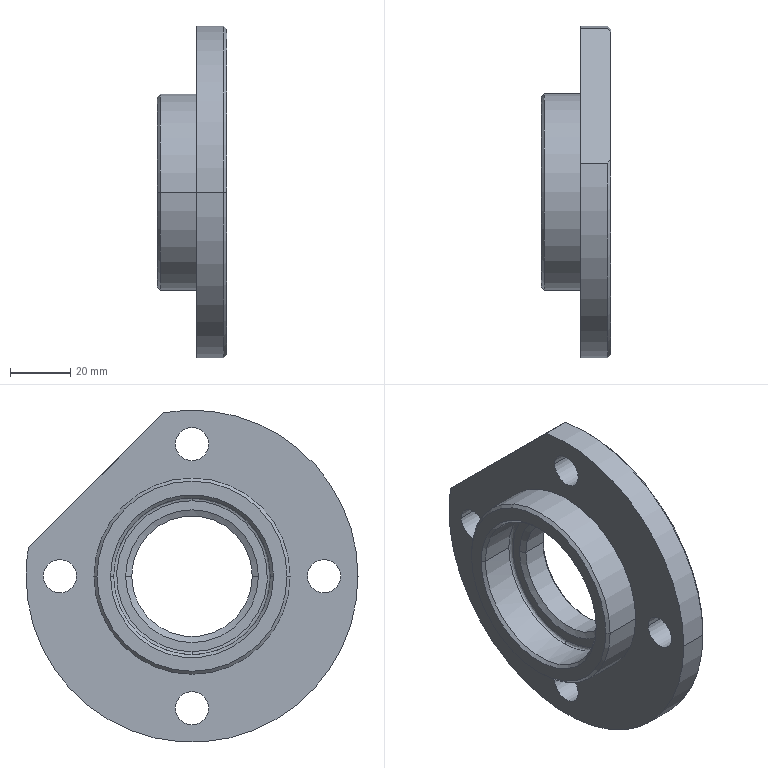Part | SolidWorks | features BaseBody 1 | 1 solid | 35 faces | box 23 x 110 x 110 mm | volume 89416 mm3 | cylinder 17 | cone 11 | plane 5 | spline 2 | commonest cylinder face diameters 11 x8 110 x3 40 x2 52 x2 65 x2